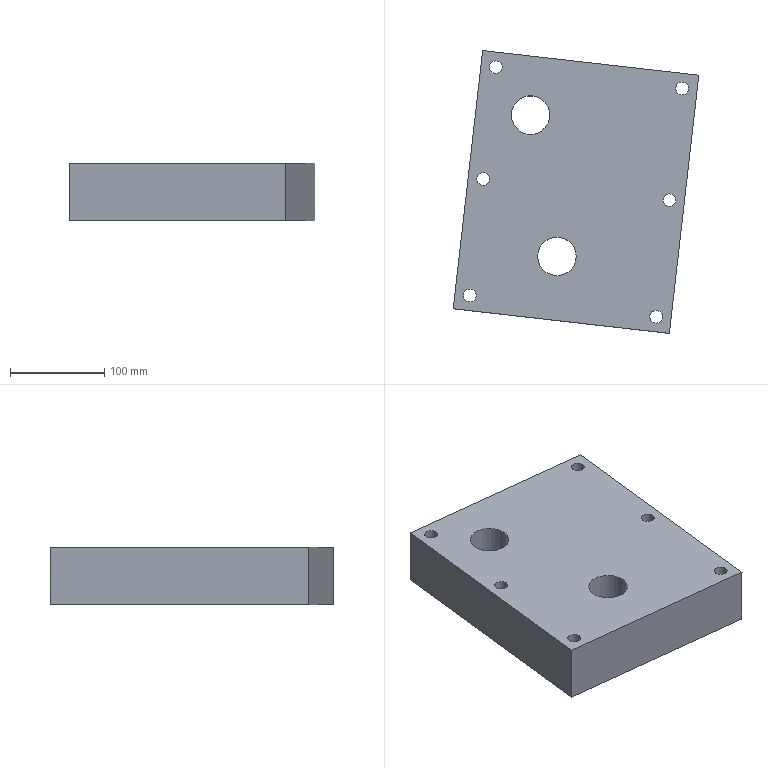Part | NX | features 7 2 | 1 solid | 60 faces | box 260.759 x 300.376 x 61 mm | volume 3148714 mm3 | cylinder 29 | plane 25 | cone 5 | spline 1 | commonest cylinder face diameters 10 x10 13.5 x6 20 x6 10.3 x5 41 x2